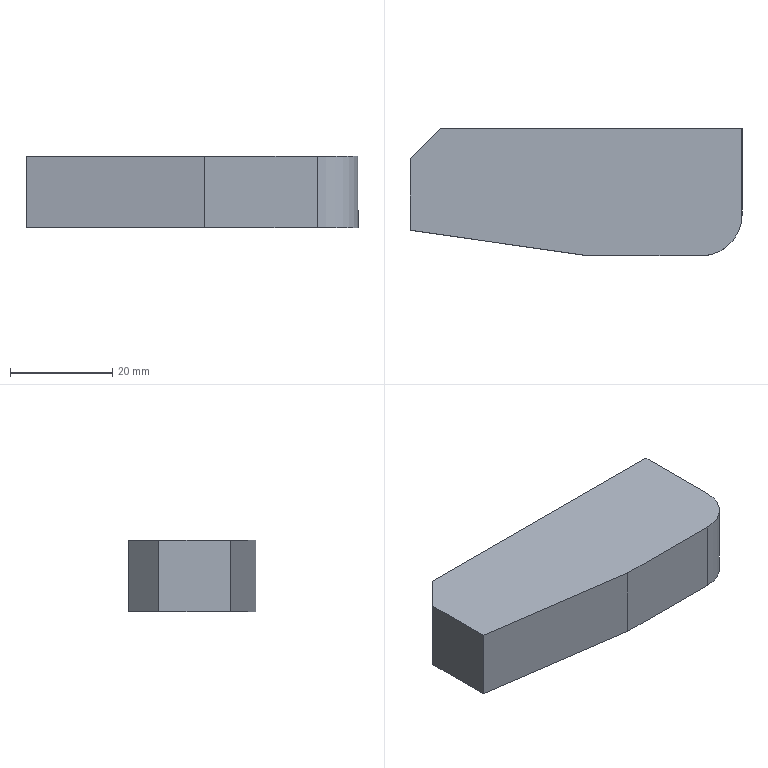Part | SolidWorks | features Chamfer 1, Extrusion 1, Fillet 1 | 1 solid | 9 faces | box 65 x 25 x 14 mm | volume 21081 mm3 | plane 8 | cylinder 1 | commonest cylinder face diameters 16 x1
STEP:
#1=CARTESIAN_POINT('',(35.,0.,-7.));
#2=VERTEX_POINT('',#1);
#3=CARTESIAN_POINT('',(57.,0.,-7.));
#4=VERTEX_POINT('',#3);
#5=CARTESIAN_POINT('',(35.,0.,-7.));
#6=DIRECTION('',(1.,0.,0.));
#7=VECTOR('',#6,1000.);
#8=LINE('',#5,#7);
#9=EDGE_CURVE('',#2,#4,#8,.T.);
#10=ORIENTED_EDGE('',*,*,#9,.T.);
#11=CARTESIAN_POINT('',(57.,0.,7.));
#12=VERTEX_POINT('',#11);
#13=CARTESIAN_POINT('',(57.,0.,7.));
#14=DIRECTION('',(0.,0.,1.));
#15=VECTOR('',#14,1000.);
#16=LINE('',#13,#15);
#17=EDGE_CURVE('',#4,#12,#16,.T.);
#18=ORIENTED_EDGE('',*,*,#17,.T.);
#19=CARTESIAN_POINT('',(35.,0.,7.));
#20=VERTEX_POINT('',#19);
#21=CARTESIAN_POINT('',(35.,0.,7.));
#22=DIRECTION('',(1.,0.,0.));
#23=VECTOR('',#22,1000.);
#24=LINE('',#21,#23);
#25=EDGE_CURVE('',#20,#12,#24,.T.);
#26=ORIENTED_EDGE('',*,*,#25,.F.);
#27=CARTESIAN_POINT('',(35.,0.,7.));
#28=DIRECTION('',(0.,0.,-1.));
#29=VECTOR('',#28,1000.);
#30=LINE('',#27,#29);
#31=EDGE_CURVE('',#20,#2,#30,.T.);
#32=ORIENTED_EDGE('',*,*,#31,.T.);
#33=EDGE_LOOP('',(#10,#18,#26,#32));
#34=FACE_OUTER_BOUND('',#33,.T.);
#35=CARTESIAN_POINT('',(35.,0.,7.));
#36=DIRECTION('',(0.,1.,0.));
#37=DIRECTION('',(0.,0.,1.));
#38=AXIS2_PLACEMENT_3D('',#35,#36,#37);
#39=PLANE('',#38);
#40=ADVANCED_FACE('',(#34),#39,.F.);
#41=CARTESIAN_POINT('',(65.,8.,7.));
#42=VERTEX_POINT('',#41);
#43=CARTESIAN_POINT('',(65.,25.,7.));
#44=VERTEX_POINT('',#43);
#45=CARTESIAN_POINT('',(65.,25.,7.));
#46=DIRECTION('',(0.,1.,0.));
#47=VECTOR('',#46,1000.);
#48=LINE('',#45,#47);
#49=EDGE_CURVE('',#42,#44,#48,.T.);
#50=ORIENTED_EDGE('',*,*,#49,.F.);
#51=CARTESIAN_POINT('',(65.,8.,-7.));
#52=VERTEX_POINT('',#51);
#53=CARTESIAN_POINT('',(65.,8.,7.));
#54=DIRECTION('',(0.,0.,-1.));
#55=VECTOR('',#54,1000.);
#56=LINE('',#53,#55);
#57=EDGE_CURVE('',#42,#52,#56,.T.);
#58=ORIENTED_EDGE('',*,*,#57,.T.);
#59=CARTESIAN_POINT('',(65.,25.,-7.));
#60=VERTEX_POINT('',#59);
#61=CARTESIAN_POINT('',(65.,25.,-7.));
#62=DIRECTION('',(0.,1.,0.));
#63=VECTOR('',#62,1000.);
#64=LINE('',#61,#63);
#65=EDGE_CURVE('',#52,#60,#64,.T.);
#66=ORIENTED_EDGE('',*,*,#65,.T.);
#67=CARTESIAN_POINT('',(65.,25.,7.));
#68=DIRECTION('',(0.,0.,-1.));
#69=VECTOR('',#68,1000.);
#70=LINE('',#67,#69);
#71=EDGE_CURVE('',#44,#60,#70,.T.);
#72=ORIENTED_EDGE('',*,*,#71,.F.);
#73=EDGE_LOOP('',(#50,#58,#66,#72));
#74=FACE_OUTER_BOUND('',#73,.T.);
#75=CARTESIAN_POINT('',(65.,25.,7.));
#76=DIRECTION('',(-1.,0.,0.));
#77=DIRECTION('',(0.,0.,1.));
#78=AXIS2_PLACEMENT_3D('',#75,#76,#77);
#79=PLANE('',#78);
#80=ADVANCED_FACE('',(#74),#79,.F.);
#81=CARTESIAN_POINT('',(6.,25.,-7.));
#82=VERTEX_POINT('',#81);
#83=CARTESIAN_POINT('',(0.,25.,-7.));
#84=DIRECTION('',(-1.,0.,0.));
#85=VECTOR('',#84,1000.);
#86=LINE('',#83,#85);
#87=EDGE_CURVE('',#60,#82,#86,.T.);
#88=ORIENTED_EDGE('',*,*,#87,.T.);
#89=CARTESIAN_POINT('',(6.,25.,7.));
#90=VERTEX_POINT('',#89);
#91=CARTESIAN_POINT('',(6.,25.,7.));
#92=DIRECTION('',(0.,0.,1.));
#93=VECTOR('',#92,1000.);
#94=LINE('',#91,#93);
#95=EDGE_CURVE('',#82,#90,#94,.T.);
#96=ORIENTED_EDGE('',*,*,#95,.T.);
#97=CARTESIAN_POINT('',(0.,25.,7.));
#98=DIRECTION('',(-1.,0.,0.));
#99=VECTOR('',#98,1000.);
#100=LINE('',#97,#99);
#101=EDGE_CURVE('',#44,#90,#100,.T.);
#102=ORIENTED_EDGE('',*,*,#101,.F.);
#103=ORIENTED_EDGE('',*,*,#71,.T.);
#104=EDGE_LOOP('',(#88,#96,#102,#103));
#105=FACE_OUTER_BOUND('',#104,.T.);
#106=CARTESIAN_POINT('',(0.,25.,7.));
#107=DIRECTION('',(0.,-1.,0.));
#108=DIRECTION('',(0.,0.,-1.));
#109=AXIS2_PLACEMENT_3D('',#106,#107,#108);
#110=PLANE('',#109);
#111=ADVANCED_FACE('',(#105),#110,.F.);
#112=CARTESIAN_POINT('',(0.,19.,7.));
#113=VERTEX_POINT('',#112);
#114=CARTESIAN_POINT('',(0.,5.,7.));
#115=VERTEX_POINT('',#114);
#116=CARTESIAN_POINT('',(0.,5.,7.));
#117=DIRECTION('',(0.,-1.,0.));
#118=VECTOR('',#117,1000.);
#119=LINE('',#116,#118);
#120=EDGE_CURVE('',#113,#115,#119,.T.);
#121=ORIENTED_EDGE('',*,*,#120,.F.);
#122=CARTESIAN_POINT('',(0.,19.,-7.));
#123=VERTEX_POINT('',#122);
#124=CARTESIAN_POINT('',(0.,19.,7.));
#125=DIRECTION('',(0.,0.,-1.));
#126=VECTOR('',#125,1000.);
#127=LINE('',#124,#126);
#128=EDGE_CURVE('',#113,#123,#127,.T.);
#129=ORIENTED_EDGE('',*,*,#128,.T.);
#130=CARTESIAN_POINT('',(0.,5.,-7.));
#131=VERTEX_POINT('',#130);
#132=CARTESIAN_POINT('',(0.,5.,-7.));
#133=DIRECTION('',(0.,-1.,0.));
#134=VECTOR('',#133,1000.);
#135=LINE('',#132,#134);
#136=EDGE_CURVE('',#123,#131,#135,.T.);
#137=ORIENTED_EDGE('',*,*,#136,.T.);
#138=CARTESIAN_POINT('',(0.,5.,7.));
#139=DIRECTION('',(0.,0.,-1.));
#140=VECTOR('',#139,1000.);
#141=LINE('',#138,#140);
#142=EDGE_CURVE('',#115,#131,#141,.T.);
#143=ORIENTED_EDGE('',*,*,#142,.F.);
#144=EDGE_LOOP('',(#121,#129,#137,#143));
#145=FACE_OUTER_BOUND('',#144,.T.);
#146=CARTESIAN_POINT('',(0.,5.,7.));
#147=DIRECTION('',(1.,0.,0.));
#148=DIRECTION('',(0.,1.,0.));
#149=AXIS2_PLACEMENT_3D('',#146,#147,#148);
#150=PLANE('',#149);
#151=ADVANCED_FACE('',(#145),#150,.F.);
#152=CARTESIAN_POINT('',(0.,5.,-7.));
#153=DIRECTION('',(0.9899,-0.1414,0.));
#154=VECTOR('',#153,1000.);
#155=LINE('',#152,#154);
#156=EDGE_CURVE('',#131,#2,#155,.T.);
#157=ORIENTED_EDGE('',*,*,#156,.T.);
#158=ORIENTED_EDGE('',*,*,#31,.F.);
#159=CARTESIAN_POINT('',(0.,5.,7.));
#160=DIRECTION('',(0.9899,-0.1414,0.));
#161=VECTOR('',#160,1000.);
#162=LINE('',#159,#161);
#163=EDGE_CURVE('',#115,#20,#162,.T.);
#164=ORIENTED_EDGE('',*,*,#163,.F.);
#165=ORIENTED_EDGE('',*,*,#142,.T.);
#166=EDGE_LOOP('',(#157,#158,#164,#165));
#167=FACE_OUTER_BOUND('',#166,.T.);
#168=CARTESIAN_POINT('',(0.,5.,7.));
#169=DIRECTION('',(0.1414,0.9899,0.));
#170=DIRECTION('',(-0.9899,0.1414,0.));
#171=AXIS2_PLACEMENT_3D('',#168,#169,#170);
#172=PLANE('',#171);
#173=ADVANCED_FACE('',(#167),#172,.F.);
#174=ORIENTED_EDGE('',*,*,#25,.T.);
#175=CARTESIAN_POINT('',(57.,8.,7.));
#176=DIRECTION('',(0.,0.,1.));
#177=DIRECTION('',(-1.,0.,0.));
#178=AXIS2_PLACEMENT_3D('',#175,#176,#177);
#179=CIRCLE('',#178,8.);
#180=EDGE_CURVE('',#12,#42,#179,.T.);
#181=ORIENTED_EDGE('',*,*,#180,.T.);
#182=ORIENTED_EDGE('',*,*,#49,.T.);
#183=ORIENTED_EDGE('',*,*,#101,.T.);
#184=CARTESIAN_POINT('',(0.,19.,7.));
#185=DIRECTION('',(-0.7071,-0.7071,0.));
#186=VECTOR('',#185,1000.);
#187=LINE('',#184,#186);
#188=EDGE_CURVE('',#90,#113,#187,.T.);
#189=ORIENTED_EDGE('',*,*,#188,.T.);
#190=ORIENTED_EDGE('',*,*,#120,.T.);
#191=ORIENTED_EDGE('',*,*,#163,.T.);
#192=EDGE_LOOP('',(#174,#181,#182,#183,#189,#190,#191));
#193=FACE_OUTER_BOUND('',#192,.T.);
#194=CARTESIAN_POINT('',(0.,0.,7.));
#195=DIRECTION('',(0.,0.,-1.));
#196=DIRECTION('',(-1.,0.,0.));
#197=AXIS2_PLACEMENT_3D('',#194,#195,#196);
#198=PLANE('',#197);
#199=ADVANCED_FACE('',(#193),#198,.F.);
#200=ORIENTED_EDGE('',*,*,#65,.F.);
#201=CARTESIAN_POINT('',(57.,8.,-7.));
#202=DIRECTION('',(0.,0.,-1.));
#203=DIRECTION('',(-1.,0.,0.));
#204=AXIS2_PLACEMENT_3D('',#201,#202,#203);
#205=CIRCLE('',#204,8.);
#206=EDGE_CURVE('',#52,#4,#205,.T.);
#207=ORIENTED_EDGE('',*,*,#206,.T.);
#208=ORIENTED_EDGE('',*,*,#9,.F.);
#209=ORIENTED_EDGE('',*,*,#156,.F.);
#210=ORIENTED_EDGE('',*,*,#136,.F.);
#211=CARTESIAN_POINT('',(-9.5,9.5,-7.));
#212=DIRECTION('',(0.7071,0.7071,0.));
#213=VECTOR('',#212,1000.);
#214=LINE('',#211,#213);
#215=EDGE_CURVE('',#123,#82,#214,.T.);
#216=ORIENTED_EDGE('',*,*,#215,.T.);
#217=ORIENTED_EDGE('',*,*,#87,.F.);
#218=EDGE_LOOP('',(#200,#207,#208,#209,#210,#216,#217));
#219=FACE_OUTER_BOUND('',#218,.T.);
#220=CARTESIAN_POINT('',(0.,0.,-7.));
#221=DIRECTION('',(0.,0.,-1.));
#222=DIRECTION('',(-1.,0.,0.));
#223=AXIS2_PLACEMENT_3D('',#220,#221,#222);
#224=PLANE('',#223);
#225=ADVANCED_FACE('',(#219),#224,.T.);
#226=ORIENTED_EDGE('',*,*,#188,.F.);
#227=ORIENTED_EDGE('',*,*,#95,.F.);
#228=ORIENTED_EDGE('',*,*,#215,.F.);
#229=ORIENTED_EDGE('',*,*,#128,.F.);
#230=EDGE_LOOP('',(#226,#227,#228,#229));
#231=FACE_OUTER_BOUND('',#230,.T.);
#232=CARTESIAN_POINT('',(0.,19.,7.));
#233=DIRECTION('',(0.7071,-0.7071,0.));
#234=DIRECTION('',(0.,0.,-1.));
#235=AXIS2_PLACEMENT_3D('',#232,#233,#234);
#236=PLANE('',#235);
#237=ADVANCED_FACE('',(#231),#236,.F.);
#238=ORIENTED_EDGE('',*,*,#180,.F.);
#239=ORIENTED_EDGE('',*,*,#17,.F.);
#240=ORIENTED_EDGE('',*,*,#206,.F.);
#241=ORIENTED_EDGE('',*,*,#57,.F.);
#242=EDGE_LOOP('',(#238,#239,#240,#241));
#243=FACE_OUTER_BOUND('',#242,.T.);
#244=CARTESIAN_POINT('',(57.,8.,7.));
#245=DIRECTION('',(0.,0.,-1.));
#246=DIRECTION('',(-1.,0.,0.));
#247=AXIS2_PLACEMENT_3D('',#244,#245,#246);
#248=CYLINDRICAL_SURFACE('',#247,8.);
#249=ADVANCED_FACE('',(#243),#248,.T.);
#250=CLOSED_SHELL('',(#40,#80,#111,#151,#173,#199,#225,#237,#249));
#251=MANIFOLD_SOLID_BREP('',#250);
#252=CARTESIAN_POINT('',(0.,0.,0.));
#253=DIRECTION('',(0.,0.,1.));
#254=DIRECTION('',(1.,0.,0.));
#255=AXIS2_PLACEMENT_3D('',#252,#253,#254);
#256=(LENGTH_UNIT()NAMED_UNIT(*)SI_UNIT(.MILLI.,.METRE.));
#257=UNCERTAINTY_MEASURE_WITH_UNIT(LENGTH_MEASURE(0.00001),#256,'','');
#258=(NAMED_UNIT(*)PLANE_ANGLE_UNIT()SI_UNIT($,.RADIAN.));
#259=(NAMED_UNIT(*)SI_UNIT($,.STERADIAN.)SOLID_ANGLE_UNIT());
#260=(GEOMETRIC_REPRESENTATION_CONTEXT(3)GLOBAL_UNCERTAINTY_ASSIGNED_CONTEXT((#257))GLOBAL_UNIT_ASSIGNED_CONTEXT((#256,#258,#259))REPRESENTATION_CONTEXT('',''));
#261=ADVANCED_BREP_SHAPE_REPRESENTATION('',(#251,#255),#260);